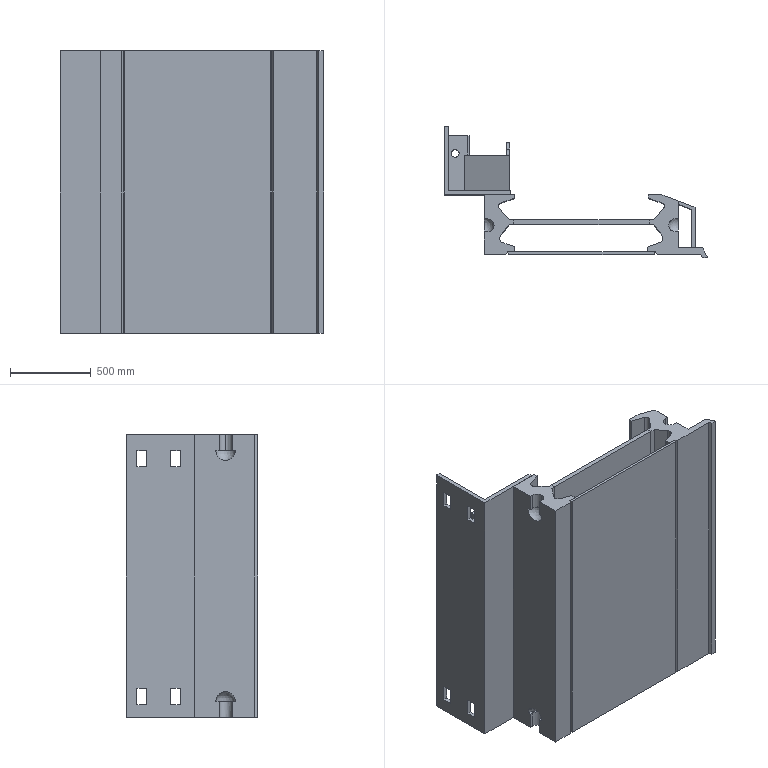Part | SolidWorks | 7 solids | 216 faces | box 1628 x 811.488 x 1750 mm | volume 332107465 mm3 | plane 156 | cylinder 52 | spline 4 | sphere 4 | commonest cylinder face diameters 80 x22 70 x14 50 x12 63.152 x4